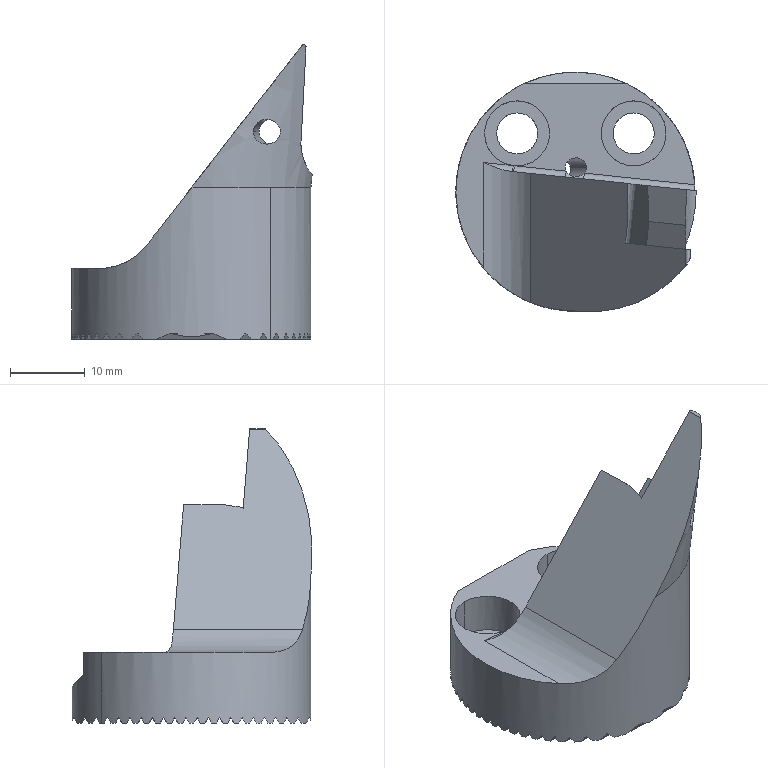Part | 1 solid | 156 faces | volume 9981 mm3 | plane 124 | cylinder 25 | cone 5 | spline 2 | commonest cylinder face diameters 5.5 x4 8.7 x4 1.6 x3 2.5 x2 3.3 x2 10.5 x2